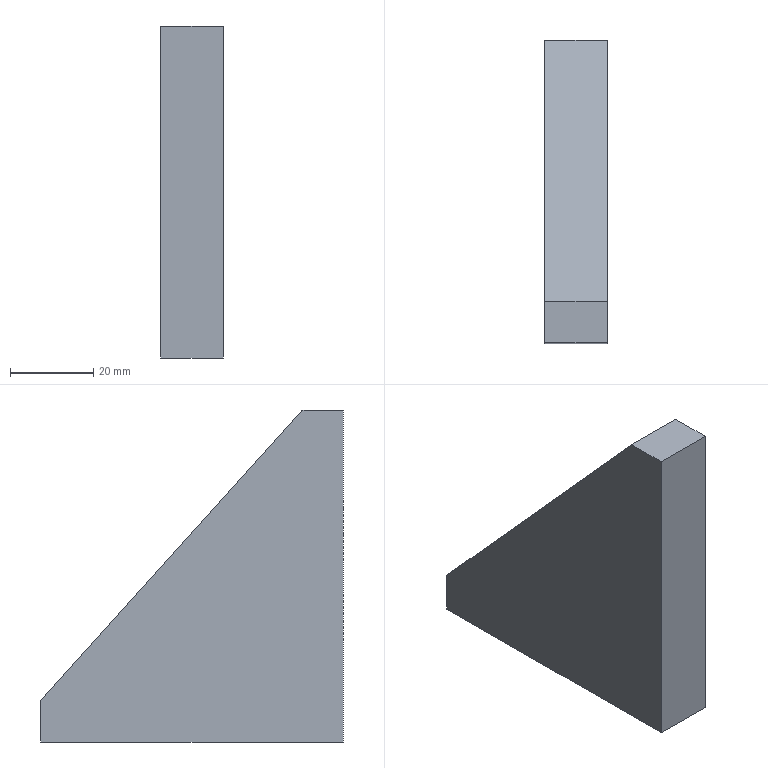Part | NX | features BREP 1, DATUM_CSYS 1 | 1 solid | 7 faces | box 15 x 73 x 80 mm | volume 54525 mm3 | plane 7
STEP:
#1=CARTESIAN_POINT('',(-24.,-57.,224.));
#2=VERTEX_POINT('',#1);
#3=CARTESIAN_POINT('',(-24.,-57.,144.));
#4=VERTEX_POINT('',#3);
#5=CARTESIAN_POINT('',(-24.,-57.,224.));
#6=DIRECTION('',(0.,0.,-1.));
#7=VECTOR('',#6,1000.);
#8=LINE('',#5,#7);
#9=EDGE_CURVE('',#2,#4,#8,.T.);
#10=ORIENTED_EDGE('',*,*,#9,.F.);
#11=CARTESIAN_POINT('',(-39.,-57.,224.));
#12=VERTEX_POINT('',#11);
#13=CARTESIAN_POINT('',(-39.,-57.,224.));
#14=DIRECTION('',(1.,0.,0.));
#15=VECTOR('',#14,1000.);
#16=LINE('',#13,#15);
#17=EDGE_CURVE('',#12,#2,#16,.T.);
#18=ORIENTED_EDGE('',*,*,#17,.F.);
#19=CARTESIAN_POINT('',(-39.,-57.,144.));
#20=VERTEX_POINT('',#19);
#21=CARTESIAN_POINT('',(-39.,-57.,224.));
#22=DIRECTION('',(0.,0.,-1.));
#23=VECTOR('',#22,1000.);
#24=LINE('',#21,#23);
#25=EDGE_CURVE('',#12,#20,#24,.T.);
#26=ORIENTED_EDGE('',*,*,#25,.T.);
#27=CARTESIAN_POINT('',(-39.,-57.,144.));
#28=DIRECTION('',(1.,0.,0.));
#29=VECTOR('',#28,1000.);
#30=LINE('',#27,#29);
#31=EDGE_CURVE('',#20,#4,#30,.T.);
#32=ORIENTED_EDGE('',*,*,#31,.T.);
#33=EDGE_LOOP('',(#10,#18,#26,#32));
#34=FACE_BOUND('',#33,.T.);
#35=CARTESIAN_POINT('',(-39.,-57.,224.));
#36=DIRECTION('',(0.,-1.,0.));
#37=DIRECTION('',(0.,0.,-1.));
#38=AXIS2_PLACEMENT_3D('',#35,#36,#37);
#39=PLANE('',#38);
#40=ADVANCED_FACE('',(#34),#39,.T.);
#41=CARTESIAN_POINT('',(-24.,16.,144.));
#42=VERTEX_POINT('',#41);
#43=CARTESIAN_POINT('',(-24.,-57.,144.));
#44=DIRECTION('',(0.,1.,0.));
#45=VECTOR('',#44,1000.);
#46=LINE('',#43,#45);
#47=EDGE_CURVE('',#4,#42,#46,.T.);
#48=ORIENTED_EDGE('',*,*,#47,.F.);
#49=ORIENTED_EDGE('',*,*,#31,.F.);
#50=CARTESIAN_POINT('',(-39.,16.,144.));
#51=VERTEX_POINT('',#50);
#52=CARTESIAN_POINT('',(-39.,-57.,144.));
#53=DIRECTION('',(0.,1.,0.));
#54=VECTOR('',#53,1000.);
#55=LINE('',#52,#54);
#56=EDGE_CURVE('',#20,#51,#55,.T.);
#57=ORIENTED_EDGE('',*,*,#56,.T.);
#58=CARTESIAN_POINT('',(-39.,16.,144.));
#59=DIRECTION('',(1.,0.,0.));
#60=VECTOR('',#59,1000.);
#61=LINE('',#58,#60);
#62=EDGE_CURVE('',#51,#42,#61,.T.);
#63=ORIENTED_EDGE('',*,*,#62,.T.);
#64=EDGE_LOOP('',(#48,#49,#57,#63));
#65=FACE_BOUND('',#64,.T.);
#66=CARTESIAN_POINT('',(-39.,-57.,144.));
#67=DIRECTION('',(0.,0.,-1.));
#68=DIRECTION('',(-1.,0.,0.));
#69=AXIS2_PLACEMENT_3D('',#66,#67,#68);
#70=PLANE('',#69);
#71=ADVANCED_FACE('',(#65),#70,.T.);
#72=CARTESIAN_POINT('',(-24.,16.,154.));
#73=VERTEX_POINT('',#72);
#74=CARTESIAN_POINT('',(-24.,16.,144.));
#75=DIRECTION('',(0.,0.,1.));
#76=VECTOR('',#75,1000.);
#77=LINE('',#74,#76);
#78=EDGE_CURVE('',#42,#73,#77,.T.);
#79=ORIENTED_EDGE('',*,*,#78,.F.);
#80=ORIENTED_EDGE('',*,*,#62,.F.);
#81=CARTESIAN_POINT('',(-39.,16.,154.));
#82=VERTEX_POINT('',#81);
#83=CARTESIAN_POINT('',(-39.,16.,144.));
#84=DIRECTION('',(0.,0.,1.));
#85=VECTOR('',#84,1000.);
#86=LINE('',#83,#85);
#87=EDGE_CURVE('',#51,#82,#86,.T.);
#88=ORIENTED_EDGE('',*,*,#87,.T.);
#89=CARTESIAN_POINT('',(-39.,16.,154.));
#90=DIRECTION('',(1.,0.,0.));
#91=VECTOR('',#90,1000.);
#92=LINE('',#89,#91);
#93=EDGE_CURVE('',#82,#73,#92,.T.);
#94=ORIENTED_EDGE('',*,*,#93,.T.);
#95=EDGE_LOOP('',(#79,#80,#88,#94));
#96=FACE_BOUND('',#95,.T.);
#97=CARTESIAN_POINT('',(-39.,16.,144.));
#98=DIRECTION('',(0.,1.,0.));
#99=DIRECTION('',(0.,0.,1.));
#100=AXIS2_PLACEMENT_3D('',#97,#98,#99);
#101=PLANE('',#100);
#102=ADVANCED_FACE('',(#96),#101,.T.);
#103=CARTESIAN_POINT('',(-24.,-47.,224.));
#104=VERTEX_POINT('',#103);
#105=CARTESIAN_POINT('',(-24.,16.,154.));
#106=DIRECTION('',(0.,-0.669,0.7433));
#107=VECTOR('',#106,1000.);
#108=LINE('',#105,#107);
#109=EDGE_CURVE('',#73,#104,#108,.T.);
#110=ORIENTED_EDGE('',*,*,#109,.F.);
#111=ORIENTED_EDGE('',*,*,#93,.F.);
#112=CARTESIAN_POINT('',(-39.,-47.,224.));
#113=VERTEX_POINT('',#112);
#114=CARTESIAN_POINT('',(-39.,16.,154.));
#115=DIRECTION('',(0.,-0.669,0.7433));
#116=VECTOR('',#115,1000.);
#117=LINE('',#114,#116);
#118=EDGE_CURVE('',#82,#113,#117,.T.);
#119=ORIENTED_EDGE('',*,*,#118,.T.);
#120=CARTESIAN_POINT('',(-39.,-47.,224.));
#121=DIRECTION('',(1.,0.,0.));
#122=VECTOR('',#121,1000.);
#123=LINE('',#120,#122);
#124=EDGE_CURVE('',#113,#104,#123,.T.);
#125=ORIENTED_EDGE('',*,*,#124,.T.);
#126=EDGE_LOOP('',(#110,#111,#119,#125));
#127=FACE_BOUND('',#126,.T.);
#128=CARTESIAN_POINT('',(-39.,16.,154.));
#129=DIRECTION('',(0.,0.7433,0.669));
#130=DIRECTION('',(0.,-0.669,0.7433));
#131=AXIS2_PLACEMENT_3D('',#128,#129,#130);
#132=PLANE('',#131);
#133=ADVANCED_FACE('',(#127),#132,.T.);
#134=CARTESIAN_POINT('',(-24.,-47.,224.));
#135=DIRECTION('',(0.,-1.,0.));
#136=VECTOR('',#135,1000.);
#137=LINE('',#134,#136);
#138=EDGE_CURVE('',#104,#2,#137,.T.);
#139=ORIENTED_EDGE('',*,*,#138,.F.);
#140=ORIENTED_EDGE('',*,*,#124,.F.);
#141=CARTESIAN_POINT('',(-39.,-47.,224.));
#142=DIRECTION('',(0.,-1.,0.));
#143=VECTOR('',#142,1000.);
#144=LINE('',#141,#143);
#145=EDGE_CURVE('',#113,#12,#144,.T.);
#146=ORIENTED_EDGE('',*,*,#145,.T.);
#147=ORIENTED_EDGE('',*,*,#17,.T.);
#148=EDGE_LOOP('',(#139,#140,#146,#147));
#149=FACE_BOUND('',#148,.T.);
#150=CARTESIAN_POINT('',(-39.,-47.,224.));
#151=DIRECTION('',(0.,0.,1.));
#152=DIRECTION('',(1.,0.,0.));
#153=AXIS2_PLACEMENT_3D('',#150,#151,#152);
#154=PLANE('',#153);
#155=ADVANCED_FACE('',(#149),#154,.T.);
#156=ORIENTED_EDGE('',*,*,#25,.F.);
#157=ORIENTED_EDGE('',*,*,#145,.F.);
#158=ORIENTED_EDGE('',*,*,#118,.F.);
#159=ORIENTED_EDGE('',*,*,#87,.F.);
#160=ORIENTED_EDGE('',*,*,#56,.F.);
#161=EDGE_LOOP('',(#156,#157,#158,#159,#160));
#162=FACE_BOUND('',#161,.T.);
#163=CARTESIAN_POINT('',(-39.,0.,0.));
#164=DIRECTION('',(1.,0.,0.));
#165=DIRECTION('',(0.,0.,-1.));
#166=AXIS2_PLACEMENT_3D('',#163,#164,#165);
#167=PLANE('',#166);
#168=ADVANCED_FACE('',(#162),#167,.F.);
#169=ORIENTED_EDGE('',*,*,#9,.T.);
#170=ORIENTED_EDGE('',*,*,#47,.T.);
#171=ORIENTED_EDGE('',*,*,#78,.T.);
#172=ORIENTED_EDGE('',*,*,#109,.T.);
#173=ORIENTED_EDGE('',*,*,#138,.T.);
#174=EDGE_LOOP('',(#169,#170,#171,#172,#173));
#175=FACE_BOUND('',#174,.T.);
#176=CARTESIAN_POINT('',(-24.,0.,0.));
#177=DIRECTION('',(1.,0.,0.));
#178=DIRECTION('',(0.,0.,-1.));
#179=AXIS2_PLACEMENT_3D('',#176,#177,#178);
#180=PLANE('',#179);
#181=ADVANCED_FACE('',(#175),#180,.T.);
#182=CLOSED_SHELL('',(#40,#71,#102,#133,#155,#168,#181));
#183=MANIFOLD_SOLID_BREP('',#182);
#184=(LENGTH_UNIT()NAMED_UNIT(*)SI_UNIT(.MILLI.,.METRE.));
#185=UNCERTAINTY_MEASURE_WITH_UNIT(LENGTH_MEASURE(0.00001),#184,'','');
#186=(NAMED_UNIT(*)PLANE_ANGLE_UNIT()SI_UNIT($,.RADIAN.));
#187=(NAMED_UNIT(*)SI_UNIT($,.STERADIAN.)SOLID_ANGLE_UNIT());
#188=(GEOMETRIC_REPRESENTATION_CONTEXT(3)GLOBAL_UNCERTAINTY_ASSIGNED_CONTEXT((#185))GLOBAL_UNIT_ASSIGNED_CONTEXT((#184,#186,#187))REPRESENTATION_CONTEXT('',''));
#189=ADVANCED_BREP_SHAPE_REPRESENTATION('',(#183),#188);